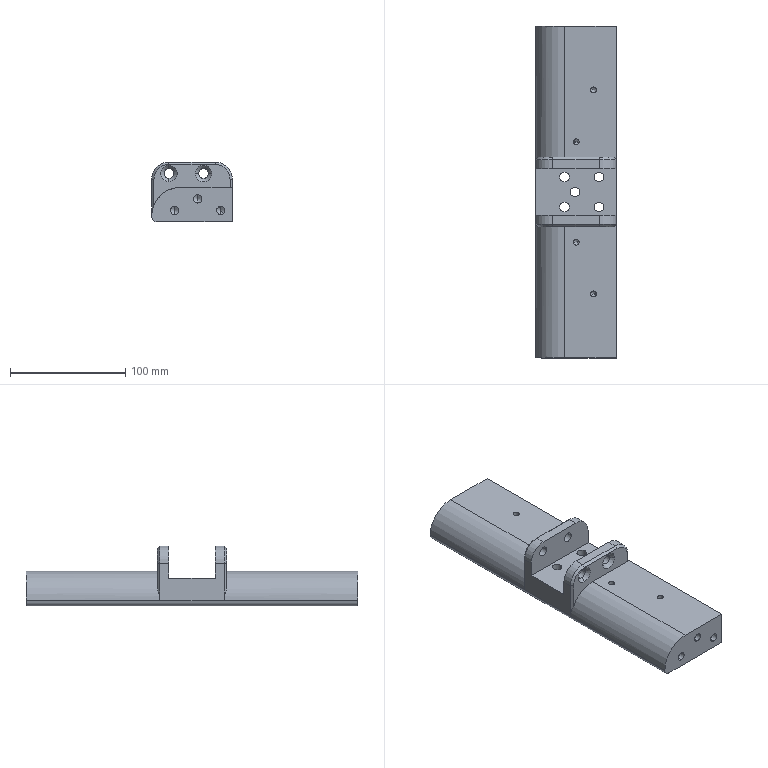Part | SolidWorks | features BaseBody 1 | 1 solid | 109 faces | box 70 x 288 x 52 mm | volume 563339 mm3 | cylinder 51 | cone 38 | plane 20 | commonest cylinder face diameters 5.2 x14 7.2 x12 8.2 x10 8.5 x8 30 x4 50 x2